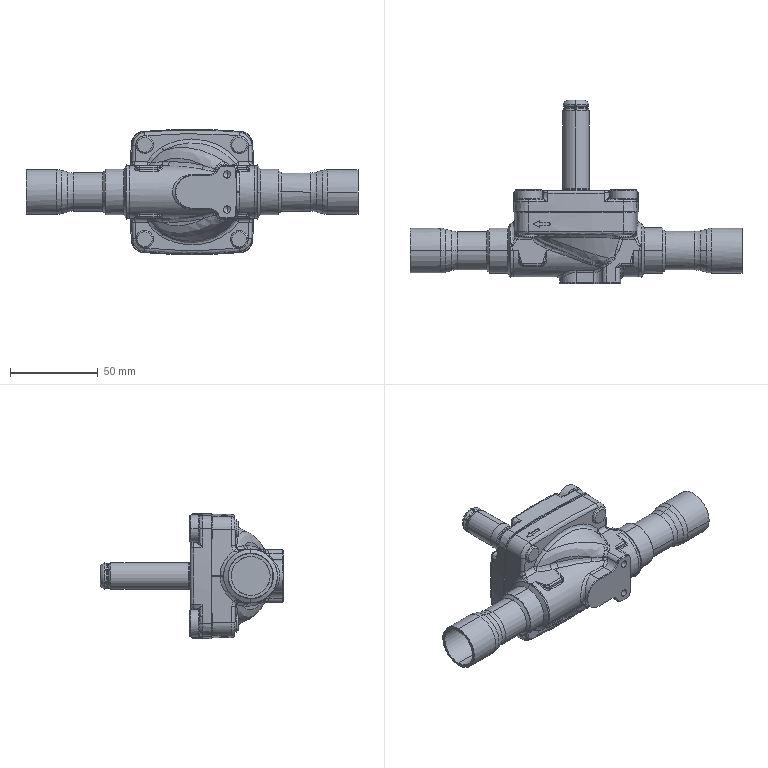Part | STEP file | seven-eighths solenoid valve | 1 solid | 884 faces | box 189.5 x 104.6 x 71.674 mm | volume 229538 mm3 | spline 370 | cylinder 232 | torus 102 | plane 100 | cone 72 | sphere 8 | commonest cylinder face diameters 1.2 x33 2.936 x29 7 x27 4 x21 10 x18 2 x16